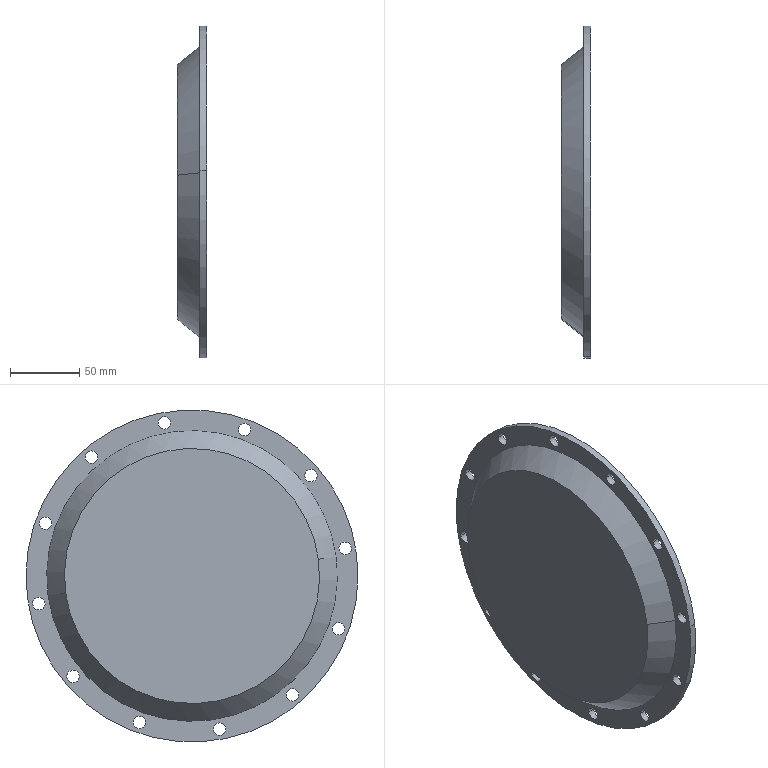Part | NX | features BREP 1 | 1 solid | 34 faces | box 21.199 x 240 x 240 mm | volume 246354 mm3 | cylinder 26 | cone 4 | plane 4 | commonest cylinder face diameters 9 x24 240 x2
STEP:
#1=CARTESIAN_POINT('',(-650.355,90.374,-73.224));
#2=VERTEX_POINT('',#1);
#3=CARTESIAN_POINT('',(-650.355,81.453,-72.035));
#4=VERTEX_POINT('',#3);
#5=CARTESIAN_POINT('',(-650.355,85.914,-72.63));
#6=DIRECTION('',(-1.,0.,0.));
#7=DIRECTION('',(0.,-0.9912,0.1321));
#8=AXIS2_PLACEMENT_3D('',#5,#6,#7);
#9=CIRCLE('',#8,4.5);
#10=EDGE_CURVE('',#2,#4,#9,.T.);
#11=ORIENTED_EDGE('',*,*,#10,.F.);
#12=CARTESIAN_POINT('',(-655.355,90.374,-73.224));
#13=VERTEX_POINT('',#12);
#14=CARTESIAN_POINT('',(-645.355,90.374,-73.224));
#15=DIRECTION('',(1.,0.,0.));
#16=VECTOR('',#15,1000.);
#17=LINE('',#14,#16);
#18=EDGE_CURVE('',#13,#2,#17,.T.);
#19=ORIENTED_EDGE('',*,*,#18,.F.);
#20=CARTESIAN_POINT('',(-655.355,81.453,-72.035));
#21=VERTEX_POINT('',#20);
#22=CARTESIAN_POINT('',(-655.355,85.914,-72.63));
#23=DIRECTION('',(-1.,0.,0.));
#24=DIRECTION('',(0.,-0.9912,0.1321));
#25=AXIS2_PLACEMENT_3D('',#22,#23,#24);
#26=CIRCLE('',#25,4.5);
#27=EDGE_CURVE('',#13,#21,#26,.T.);
#28=ORIENTED_EDGE('',*,*,#27,.T.);
#29=CARTESIAN_POINT('',(-645.355,81.453,-72.035));
#30=DIRECTION('',(1.,0.,0.));
#31=VECTOR('',#30,1000.);
#32=LINE('',#29,#31);
#33=EDGE_CURVE('',#21,#4,#32,.T.);
#34=ORIENTED_EDGE('',*,*,#33,.T.);
#35=EDGE_LOOP('',(#11,#19,#28,#34));
#36=FACE_BOUND('',#35,.T.);
#37=CARTESIAN_POINT('',(-645.355,85.914,-72.63));
#38=DIRECTION('',(-1.,0.,0.));
#39=DIRECTION('',(0.,-0.9912,0.1321));
#40=AXIS2_PLACEMENT_3D('',#37,#38,#39);
#41=CYLINDRICAL_SURFACE('',#40,4.5);
#42=ADVANCED_FACE('',(#36),#41,.F.);
#43=CARTESIAN_POINT('',(-650.355,115.179,-20.537));
#44=VERTEX_POINT('',#43);
#45=CARTESIAN_POINT('',(-650.355,106.258,-19.348));
#46=VERTEX_POINT('',#45);
#47=CARTESIAN_POINT('',(-650.355,110.718,-19.942));
#48=DIRECTION('',(-1.,0.,0.));
#49=DIRECTION('',(0.,-0.9912,0.1321));
#50=AXIS2_PLACEMENT_3D('',#47,#48,#49);
#51=CIRCLE('',#50,4.5);
#52=EDGE_CURVE('',#44,#46,#51,.T.);
#53=ORIENTED_EDGE('',*,*,#52,.F.);
#54=CARTESIAN_POINT('',(-655.355,115.179,-20.537));
#55=VERTEX_POINT('',#54);
#56=CARTESIAN_POINT('',(-645.355,115.179,-20.537));
#57=DIRECTION('',(1.,0.,0.));
#58=VECTOR('',#57,1000.);
#59=LINE('',#56,#58);
#60=EDGE_CURVE('',#55,#44,#59,.T.);
#61=ORIENTED_EDGE('',*,*,#60,.F.);
#62=CARTESIAN_POINT('',(-655.355,106.258,-19.348));
#63=VERTEX_POINT('',#62);
#64=CARTESIAN_POINT('',(-655.355,110.718,-19.942));
#65=DIRECTION('',(-1.,0.,0.));
#66=DIRECTION('',(0.,-0.9912,0.1321));
#67=AXIS2_PLACEMENT_3D('',#64,#65,#66);
#68=CIRCLE('',#67,4.5);
#69=EDGE_CURVE('',#55,#63,#68,.T.);
#70=ORIENTED_EDGE('',*,*,#69,.T.);
#71=CARTESIAN_POINT('',(-645.355,106.258,-19.348));
#72=DIRECTION('',(1.,0.,0.));
#73=VECTOR('',#72,1000.);
#74=LINE('',#71,#73);
#75=EDGE_CURVE('',#63,#46,#74,.T.);
#76=ORIENTED_EDGE('',*,*,#75,.T.);
#77=EDGE_LOOP('',(#53,#61,#70,#76));
#78=FACE_BOUND('',#77,.T.);
#79=CARTESIAN_POINT('',(-645.355,110.718,-19.942));
#80=DIRECTION('',(-1.,0.,0.));
#81=DIRECTION('',(0.,-0.9912,0.1321));
#82=AXIS2_PLACEMENT_3D('',#79,#80,#81);
#83=CYLINDRICAL_SURFACE('',#82,4.5);
#84=ADVANCED_FACE('',(#78),#83,.F.);
#85=CARTESIAN_POINT('',(-650.355,110.317,37.494));
#86=VERTEX_POINT('',#85);
#87=CARTESIAN_POINT('',(-650.355,101.396,38.683));
#88=VERTEX_POINT('',#87);
#89=CARTESIAN_POINT('',(-650.355,105.856,38.088));
#90=DIRECTION('',(-1.,0.,0.));
#91=DIRECTION('',(0.,-0.9912,0.1321));
#92=AXIS2_PLACEMENT_3D('',#89,#90,#91);
#93=CIRCLE('',#92,4.5);
#94=EDGE_CURVE('',#86,#88,#93,.T.);
#95=ORIENTED_EDGE('',*,*,#94,.F.);
#96=CARTESIAN_POINT('',(-655.355,110.317,37.494));
#97=VERTEX_POINT('',#96);
#98=CARTESIAN_POINT('',(-645.355,110.317,37.494));
#99=DIRECTION('',(1.,0.,0.));
#100=VECTOR('',#99,1000.);
#101=LINE('',#98,#100);
#102=EDGE_CURVE('',#97,#86,#101,.T.);
#103=ORIENTED_EDGE('',*,*,#102,.F.);
#104=CARTESIAN_POINT('',(-655.355,101.396,38.683));
#105=VERTEX_POINT('',#104);
#106=CARTESIAN_POINT('',(-655.355,105.856,38.088));
#107=DIRECTION('',(-1.,0.,0.));
#108=DIRECTION('',(0.,-0.9912,0.1321));
#109=AXIS2_PLACEMENT_3D('',#106,#107,#108);
#110=CIRCLE('',#109,4.5);
#111=EDGE_CURVE('',#97,#105,#110,.T.);
#112=ORIENTED_EDGE('',*,*,#111,.T.);
#113=CARTESIAN_POINT('',(-645.355,101.396,38.683));
#114=DIRECTION('',(1.,0.,0.));
#115=VECTOR('',#114,1000.);
#116=LINE('',#113,#115);
#117=EDGE_CURVE('',#105,#88,#116,.T.);
#118=ORIENTED_EDGE('',*,*,#117,.T.);
#119=EDGE_LOOP('',(#95,#103,#112,#118));
#120=FACE_BOUND('',#119,.T.);
#121=CARTESIAN_POINT('',(-645.355,105.856,38.088));
#122=DIRECTION('',(-1.,0.,0.));
#123=DIRECTION('',(0.,-0.9912,0.1321));
#124=AXIS2_PLACEMENT_3D('',#121,#122,#123);
#125=CYLINDRICAL_SURFACE('',#124,4.5);
#126=ADVANCED_FACE('',(#120),#125,.F.);
#127=CARTESIAN_POINT('',(-650.355,77.09,85.319));
#128=VERTEX_POINT('',#127);
#129=CARTESIAN_POINT('',(-650.355,68.169,86.508));
#130=VERTEX_POINT('',#129);
#131=CARTESIAN_POINT('',(-650.355,72.63,85.914));
#132=DIRECTION('',(-1.,0.,0.));
#133=DIRECTION('',(0.,-0.9912,0.1321));
#134=AXIS2_PLACEMENT_3D('',#131,#132,#133);
#135=CIRCLE('',#134,4.5);
#136=EDGE_CURVE('',#128,#130,#135,.T.);
#137=ORIENTED_EDGE('',*,*,#136,.F.);
#138=CARTESIAN_POINT('',(-655.355,77.09,85.319));
#139=VERTEX_POINT('',#138);
#140=CARTESIAN_POINT('',(-645.355,77.09,85.319));
#141=DIRECTION('',(1.,0.,0.));
#142=VECTOR('',#141,1000.);
#143=LINE('',#140,#142);
#144=EDGE_CURVE('',#139,#128,#143,.T.);
#145=ORIENTED_EDGE('',*,*,#144,.F.);
#146=CARTESIAN_POINT('',(-655.355,68.169,86.508));
#147=VERTEX_POINT('',#146);
#148=CARTESIAN_POINT('',(-655.355,72.63,85.914));
#149=DIRECTION('',(-1.,0.,0.));
#150=DIRECTION('',(0.,-0.9912,0.1321));
#151=AXIS2_PLACEMENT_3D('',#148,#149,#150);
#152=CIRCLE('',#151,4.5);
#153=EDGE_CURVE('',#139,#147,#152,.T.);
#154=ORIENTED_EDGE('',*,*,#153,.T.);
#155=CARTESIAN_POINT('',(-645.355,68.169,86.508));
#156=DIRECTION('',(1.,0.,0.));
#157=VECTOR('',#156,1000.);
#158=LINE('',#155,#157);
#159=EDGE_CURVE('',#147,#130,#158,.T.);
#160=ORIENTED_EDGE('',*,*,#159,.T.);
#161=EDGE_LOOP('',(#137,#145,#154,#160));
#162=FACE_BOUND('',#161,.T.);
#163=CARTESIAN_POINT('',(-645.355,72.63,85.914));
#164=DIRECTION('',(-1.,0.,0.));
#165=DIRECTION('',(0.,-0.9912,0.1321));
#166=AXIS2_PLACEMENT_3D('',#163,#164,#165);
#167=CYLINDRICAL_SURFACE('',#166,4.5);
#168=ADVANCED_FACE('',(#162),#167,.F.);
#169=CARTESIAN_POINT('',(-650.355,24.403,110.124));
#170=VERTEX_POINT('',#169);
#171=CARTESIAN_POINT('',(-650.355,15.482,111.313));
#172=VERTEX_POINT('',#171);
#173=CARTESIAN_POINT('',(-650.355,19.942,110.718));
#174=DIRECTION('',(-1.,0.,0.));
#175=DIRECTION('',(0.,-0.9912,0.1321));
#176=AXIS2_PLACEMENT_3D('',#173,#174,#175);
#177=CIRCLE('',#176,4.5);
#178=EDGE_CURVE('',#170,#172,#177,.T.);
#179=ORIENTED_EDGE('',*,*,#178,.F.);
#180=CARTESIAN_POINT('',(-655.355,24.403,110.124));
#181=VERTEX_POINT('',#180);
#182=CARTESIAN_POINT('',(-645.355,24.403,110.124));
#183=DIRECTION('',(1.,0.,0.));
#184=VECTOR('',#183,1000.);
#185=LINE('',#182,#184);
#186=EDGE_CURVE('',#181,#170,#185,.T.);
#187=ORIENTED_EDGE('',*,*,#186,.F.);
#188=CARTESIAN_POINT('',(-655.355,15.482,111.313));
#189=VERTEX_POINT('',#188);
#190=CARTESIAN_POINT('',(-655.355,19.942,110.718));
#191=DIRECTION('',(-1.,0.,0.));
#192=DIRECTION('',(0.,-0.9912,0.1321));
#193=AXIS2_PLACEMENT_3D('',#190,#191,#192);
#194=CIRCLE('',#193,4.5);
#195=EDGE_CURVE('',#181,#189,#194,.T.);
#196=ORIENTED_EDGE('',*,*,#195,.T.);
#197=CARTESIAN_POINT('',(-645.355,15.482,111.313));
#198=DIRECTION('',(1.,0.,0.));
#199=VECTOR('',#198,1000.);
#200=LINE('',#197,#199);
#201=EDGE_CURVE('',#189,#172,#200,.T.);
#202=ORIENTED_EDGE('',*,*,#201,.T.);
#203=EDGE_LOOP('',(#179,#187,#196,#202));
#204=FACE_BOUND('',#203,.T.);
#205=CARTESIAN_POINT('',(-645.355,19.942,110.718));
#206=DIRECTION('',(-1.,0.,0.));
#207=DIRECTION('',(0.,-0.9912,0.1321));
#208=AXIS2_PLACEMENT_3D('',#205,#206,#207);
#209=CYLINDRICAL_SURFACE('',#208,4.5);
#210=ADVANCED_FACE('',(#204),#209,.F.);
#211=CARTESIAN_POINT('',(-650.355,-33.628,105.262));
#212=VERTEX_POINT('',#211);
#213=CARTESIAN_POINT('',(-650.355,-42.549,106.451));
#214=VERTEX_POINT('',#213);
#215=CARTESIAN_POINT('',(-650.355,-38.088,105.856));
#216=DIRECTION('',(-1.,0.,0.));
#217=DIRECTION('',(0.,-0.9912,0.1321));
#218=AXIS2_PLACEMENT_3D('',#215,#216,#217);
#219=CIRCLE('',#218,4.5);
#220=EDGE_CURVE('',#212,#214,#219,.T.);
#221=ORIENTED_EDGE('',*,*,#220,.F.);
#222=CARTESIAN_POINT('',(-655.355,-33.628,105.262));
#223=VERTEX_POINT('',#222);
#224=CARTESIAN_POINT('',(-645.355,-33.628,105.262));
#225=DIRECTION('',(1.,0.,0.));
#226=VECTOR('',#225,1000.);
#227=LINE('',#224,#226);
#228=EDGE_CURVE('',#223,#212,#227,.T.);
#229=ORIENTED_EDGE('',*,*,#228,.F.);
#230=CARTESIAN_POINT('',(-655.355,-42.549,106.451));
#231=VERTEX_POINT('',#230);
#232=CARTESIAN_POINT('',(-655.355,-38.088,105.856));
#233=DIRECTION('',(-1.,0.,0.));
#234=DIRECTION('',(0.,-0.9912,0.1321));
#235=AXIS2_PLACEMENT_3D('',#232,#233,#234);
#236=CIRCLE('',#235,4.5);
#237=EDGE_CURVE('',#223,#231,#236,.T.);
#238=ORIENTED_EDGE('',*,*,#237,.T.);
#239=CARTESIAN_POINT('',(-645.355,-42.549,106.451));
#240=DIRECTION('',(1.,0.,0.));
#241=VECTOR('',#240,1000.);
#242=LINE('',#239,#241);
#243=EDGE_CURVE('',#231,#214,#242,.T.);
#244=ORIENTED_EDGE('',*,*,#243,.T.);
#245=EDGE_LOOP('',(#221,#229,#238,#244));
#246=FACE_BOUND('',#245,.T.);
#247=CARTESIAN_POINT('',(-645.355,-38.088,105.856));
#248=DIRECTION('',(-1.,0.,0.));
#249=DIRECTION('',(0.,-0.9912,0.1321));
#250=AXIS2_PLACEMENT_3D('',#247,#248,#249);
#251=CYLINDRICAL_SURFACE('',#250,4.5);
#252=ADVANCED_FACE('',(#246),#251,.F.);
#253=CARTESIAN_POINT('',(-650.355,-81.453,72.035));
#254=VERTEX_POINT('',#253);
#255=CARTESIAN_POINT('',(-650.355,-90.374,73.224));
#256=VERTEX_POINT('',#255);
#257=CARTESIAN_POINT('',(-650.355,-85.914,72.63));
#258=DIRECTION('',(-1.,0.,0.));
#259=DIRECTION('',(0.,-0.9912,0.1321));
#260=AXIS2_PLACEMENT_3D('',#257,#258,#259);
#261=CIRCLE('',#260,4.5);
#262=EDGE_CURVE('',#254,#256,#261,.T.);
#263=ORIENTED_EDGE('',*,*,#262,.F.);
#264=CARTESIAN_POINT('',(-655.355,-81.453,72.035));
#265=VERTEX_POINT('',#264);
#266=CARTESIAN_POINT('',(-645.355,-81.453,72.035));
#267=DIRECTION('',(1.,0.,0.));
#268=VECTOR('',#267,1000.);
#269=LINE('',#266,#268);
#270=EDGE_CURVE('',#265,#254,#269,.T.);
#271=ORIENTED_EDGE('',*,*,#270,.F.);
#272=CARTESIAN_POINT('',(-655.355,-90.374,73.224));
#273=VERTEX_POINT('',#272);
#274=CARTESIAN_POINT('',(-655.355,-85.914,72.63));
#275=DIRECTION('',(-1.,0.,0.));
#276=DIRECTION('',(0.,-0.9912,0.1321));
#277=AXIS2_PLACEMENT_3D('',#274,#275,#276);
#278=CIRCLE('',#277,4.5);
#279=EDGE_CURVE('',#265,#273,#278,.T.);
#280=ORIENTED_EDGE('',*,*,#279,.T.);
#281=CARTESIAN_POINT('',(-645.355,-90.374,73.224));
#282=DIRECTION('',(1.,0.,0.));
#283=VECTOR('',#282,1000.);
#284=LINE('',#281,#283);
#285=EDGE_CURVE('',#273,#256,#284,.T.);
#286=ORIENTED_EDGE('',*,*,#285,.T.);
#287=EDGE_LOOP('',(#263,#271,#280,#286));
#288=FACE_BOUND('',#287,.T.);
#289=CARTESIAN_POINT('',(-645.355,-85.914,72.63));
#290=DIRECTION('',(-1.,0.,0.));
#291=DIRECTION('',(0.,-0.9912,0.1321));
#292=AXIS2_PLACEMENT_3D('',#289,#290,#291);
#293=CYLINDRICAL_SURFACE('',#292,4.5);
#294=ADVANCED_FACE('',(#288),#293,.F.);
#295=CARTESIAN_POINT('',(-650.355,-106.258,19.348));
#296=VERTEX_POINT('',#295);
#297=CARTESIAN_POINT('',(-650.355,-115.179,20.537));
#298=VERTEX_POINT('',#297);
#299=CARTESIAN_POINT('',(-650.355,-110.718,19.942));
#300=DIRECTION('',(-1.,0.,0.));
#301=DIRECTION('',(0.,-0.9912,0.1321));
#302=AXIS2_PLACEMENT_3D('',#299,#300,#301);
#303=CIRCLE('',#302,4.5);
#304=EDGE_CURVE('',#296,#298,#303,.T.);
#305=ORIENTED_EDGE('',*,*,#304,.F.);
#306=CARTESIAN_POINT('',(-655.355,-106.258,19.348));
#307=VERTEX_POINT('',#306);
#308=CARTESIAN_POINT('',(-645.355,-106.258,19.348));
#309=DIRECTION('',(1.,0.,0.));
#310=VECTOR('',#309,1000.);
#311=LINE('',#308,#310);
#312=EDGE_CURVE('',#307,#296,#311,.T.);
#313=ORIENTED_EDGE('',*,*,#312,.F.);
#314=CARTESIAN_POINT('',(-655.355,-115.179,20.537));
#315=VERTEX_POINT('',#314);
#316=CARTESIAN_POINT('',(-655.355,-110.718,19.942));
#317=DIRECTION('',(-1.,0.,0.));
#318=DIRECTION('',(0.,-0.9912,0.1321));
#319=AXIS2_PLACEMENT_3D('',#316,#317,#318);
#320=CIRCLE('',#319,4.5);
#321=EDGE_CURVE('',#307,#315,#320,.T.);
#322=ORIENTED_EDGE('',*,*,#321,.T.);
#323=CARTESIAN_POINT('',(-645.355,-115.179,20.537));
#324=DIRECTION('',(1.,0.,0.));
#325=VECTOR('',#324,1000.);
#326=LINE('',#323,#325);
#327=EDGE_CURVE('',#315,#298,#326,.T.);
#328=ORIENTED_EDGE('',*,*,#327,.T.);
#329=EDGE_LOOP('',(#305,#313,#322,#328));
#330=FACE_BOUND('',#329,.T.);
#331=CARTESIAN_POINT('',(-645.355,-110.718,19.942));
#332=DIRECTION('',(-1.,0.,0.));
#333=DIRECTION('',(0.,-0.9912,0.1321));
#334=AXIS2_PLACEMENT_3D('',#331,#332,#333);
#335=CYLINDRICAL_SURFACE('',#334,4.5);
#336=ADVANCED_FACE('',(#330),#335,.F.);
#337=CARTESIAN_POINT('',(-650.355,-101.396,-38.683));
#338=VERTEX_POINT('',#337);
#339=CARTESIAN_POINT('',(-650.355,-110.317,-37.494));
#340=VERTEX_POINT('',#339);
#341=CARTESIAN_POINT('',(-650.355,-105.856,-38.088));
#342=DIRECTION('',(-1.,0.,0.));
#343=DIRECTION('',(0.,-0.9912,0.1321));
#344=AXIS2_PLACEMENT_3D('',#341,#342,#343);
#345=CIRCLE('',#344,4.5);
#346=EDGE_CURVE('',#338,#340,#345,.T.);
#347=ORIENTED_EDGE('',*,*,#346,.F.);
#348=CARTESIAN_POINT('',(-655.355,-101.396,-38.683));
#349=VERTEX_POINT('',#348);
#350=CARTESIAN_POINT('',(-645.355,-101.396,-38.683));
#351=DIRECTION('',(1.,0.,0.));
#352=VECTOR('',#351,1000.);
#353=LINE('',#350,#352);
#354=EDGE_CURVE('',#349,#338,#353,.T.);
#355=ORIENTED_EDGE('',*,*,#354,.F.);
#356=CARTESIAN_POINT('',(-655.355,-110.317,-37.494));
#357=VERTEX_POINT('',#356);
#358=CARTESIAN_POINT('',(-655.355,-105.856,-38.088));
#359=DIRECTION('',(-1.,0.,0.));
#360=DIRECTION('',(0.,-0.9912,0.1321));
#361=AXIS2_PLACEMENT_3D('',#358,#359,#360);
#362=CIRCLE('',#361,4.5);
#363=EDGE_CURVE('',#349,#357,#362,.T.);
#364=ORIENTED_EDGE('',*,*,#363,.T.);
#365=CARTESIAN_POINT('',(-645.355,-110.317,-37.494));
#366=DIRECTION('',(1.,0.,0.));
#367=VECTOR('',#366,1000.);
#368=LINE('',#365,#367);
#369=EDGE_CURVE('',#357,#340,#368,.T.);
#370=ORIENTED_EDGE('',*,*,#369,.T.);
#371=EDGE_LOOP('',(#347,#355,#364,#370));
#372=FACE_BOUND('',#371,.T.);
#373=CARTESIAN_POINT('',(-645.355,-105.856,-38.088));
#374=DIRECTION('',(-1.,0.,0.));
#375=DIRECTION('',(0.,-0.9912,0.1321));
#376=AXIS2_PLACEMENT_3D('',#373,#374,#375);
#377=CYLINDRICAL_SURFACE('',#376,4.5);
#378=ADVANCED_FACE('',(#372),#377,.F.);
#379=CARTESIAN_POINT('',(-650.355,-68.169,-86.508));
#380=VERTEX_POINT('',#379);
#381=CARTESIAN_POINT('',(-650.355,-77.09,-85.319));
#382=VERTEX_POINT('',#381);
#383=CARTESIAN_POINT('',(-650.355,-72.63,-85.914));
#384=DIRECTION('',(-1.,0.,0.));
#385=DIRECTION('',(0.,-0.9912,0.1321));
#386=AXIS2_PLACEMENT_3D('',#383,#384,#385);
#387=CIRCLE('',#386,4.5);
#388=EDGE_CURVE('',#380,#382,#387,.T.);
#389=ORIENTED_EDGE('',*,*,#388,.F.);
#390=CARTESIAN_POINT('',(-655.355,-68.169,-86.508));
#391=VERTEX_POINT('',#390);
#392=CARTESIAN_POINT('',(-645.355,-68.169,-86.508));
#393=DIRECTION('',(1.,0.,0.));
#394=VECTOR('',#393,1000.);
#395=LINE('',#392,#394);
#396=EDGE_CURVE('',#391,#380,#395,.T.);
#397=ORIENTED_EDGE('',*,*,#396,.F.);
#398=CARTESIAN_POINT('',(-655.355,-77.09,-85.319));
#399=VERTEX_POINT('',#398);
#400=CARTESIAN_POINT('',(-655.355,-72.63,-85.914));
#401=DIRECTION('',(-1.,0.,0.));
#402=DIRECTION('',(0.,-0.9912,0.1321));
#403=AXIS2_PLACEMENT_3D('',#400,#401,#402);
#404=CIRCLE('',#403,4.5);
#405=EDGE_CURVE('',#391,#399,#404,.T.);
#406=ORIENTED_EDGE('',*,*,#405,.T.);
#407=CARTESIAN_POINT('',(-645.355,-77.09,-85.319));
#408=DIRECTION('',(1.,0.,0.));
#409=VECTOR('',#408,1000.);
#410=LINE('',#407,#409);
#411=EDGE_CURVE('',#399,#382,#410,.T.);
#412=ORIENTED_EDGE('',*,*,#411,.T.);
#413=EDGE_LOOP('',(#389,#397,#406,#412));
#414=FACE_BOUND('',#413,.T.);
#415=CARTESIAN_POINT('',(-645.355,-72.63,-85.914));
#416=DIRECTION('',(-1.,0.,0.));
#417=DIRECTION('',(0.,-0.9912,0.1321));
#418=AXIS2_PLACEMENT_3D('',#415,#416,#417);
#419=CYLINDRICAL_SURFACE('',#418,4.5);
#420=ADVANCED_FACE('',(#414),#419,.F.);
#421=CARTESIAN_POINT('',(-650.355,-15.482,-111.313));
#422=VERTEX_POINT('',#421);
#423=CARTESIAN_POINT('',(-650.355,-24.403,-110.124));
#424=VERTEX_POINT('',#423);
#425=CARTESIAN_POINT('',(-650.355,-19.942,-110.718));
#426=DIRECTION('',(-1.,0.,0.));
#427=DIRECTION('',(0.,-0.9912,0.1321));
#428=AXIS2_PLACEMENT_3D('',#425,#426,#427);
#429=CIRCLE('',#428,4.5);
#430=EDGE_CURVE('',#422,#424,#429,.T.);
#431=ORIENTED_EDGE('',*,*,#430,.F.);
#432=CARTESIAN_POINT('',(-655.355,-15.482,-111.313));
#433=VERTEX_POINT('',#432);
#434=CARTESIAN_POINT('',(-645.355,-15.482,-111.313));
#435=DIRECTION('',(1.,0.,0.));
#436=VECTOR('',#435,1000.);
#437=LINE('',#434,#436);
#438=EDGE_CURVE('',#433,#422,#437,.T.);
#439=ORIENTED_EDGE('',*,*,#438,.F.);
#440=CARTESIAN_POINT('',(-655.355,-24.403,-110.124));
#441=VERTEX_POINT('',#440);
#442=CARTESIAN_POINT('',(-655.355,-19.942,-110.718));
#443=DIRECTION('',(-1.,0.,0.));
#444=DIRECTION('',(0.,-0.9912,0.1321));
#445=AXIS2_PLACEMENT_3D('',#442,#443,#444);
#446=CIRCLE('',#445,4.5);
#447=EDGE_CURVE('',#433,#441,#446,.T.);
#448=ORIENTED_EDGE('',*,*,#447,.T.);
#449=CARTESIAN_POINT('',(-645.355,-24.403,-110.124));
#450=DIRECTION('',(1.,0.,0.));
#451=VECTOR('',#450,1000.);
#452=LINE('',#449,#451);
#453=EDGE_CURVE('',#441,#424,#452,.T.);
#454=ORIENTED_EDGE('',*,*,#453,.T.);
#455=EDGE_LOOP('',(#431,#439,#448,#454));
#456=FACE_BOUND('',#455,.T.);
#457=CARTESIAN_POINT('',(-645.355,-19.942,-110.718));
#458=DIRECTION('',(-1.,0.,0.));
#459=DIRECTION('',(0.,-0.9912,0.1321));
#460=AXIS2_PLACEMENT_3D('',#457,#458,#459);
#461=CYLINDRICAL_SURFACE('',#460,4.5);
#462=ADVANCED_FACE('',(#456),#461,.F.);
#463=CARTESIAN_POINT('',(-650.355,42.549,-106.451));
#464=VERTEX_POINT('',#463);
#465=CARTESIAN_POINT('',(-650.355,33.628,-105.262));
#466=VERTEX_POINT('',#465);
#467=CARTESIAN_POINT('',(-650.355,38.088,-105.856));
#468=DIRECTION('',(-1.,0.,0.));
#469=DIRECTION('',(0.,-0.9912,0.1321));
#470=AXIS2_PLACEMENT_3D('',#467,#468,#469);
#471=CIRCLE('',#470,4.5);
#472=EDGE_CURVE('',#464,#466,#471,.T.);
#473=ORIENTED_EDGE('',*,*,#472,.F.);
#474=CARTESIAN_POINT('',(-655.355,42.549,-106.451));
#475=VERTEX_POINT('',#474);
#476=CARTESIAN_POINT('',(-645.355,42.549,-106.451));
#477=DIRECTION('',(1.,0.,0.));
#478=VECTOR('',#477,1000.);
#479=LINE('',#476,#478);
#480=EDGE_CURVE('',#475,#464,#479,.T.);
#481=ORIENTED_EDGE('',*,*,#480,.F.);
#482=CARTESIAN_POINT('',(-655.355,33.628,-105.262));
#483=VERTEX_POINT('',#482);
#484=CARTESIAN_POINT('',(-655.355,38.088,-105.856));
#485=DIRECTION('',(-1.,0.,0.));
#486=DIRECTION('',(0.,-0.9912,0.1321));
#487=AXIS2_PLACEMENT_3D('',#484,#485,#486);
#488=CIRCLE('',#487,4.5);
#489=EDGE_CURVE('',#475,#483,#488,.T.);
#490=ORIENTED_EDGE('',*,*,#489,.T.);
#491=CARTESIAN_POINT('',(-645.355,33.628,-105.262));
#492=DIRECTION('',(1.,0.,0.));
#493=VECTOR('',#492,1000.);
#494=LINE('',#491,#493);
#495=EDGE_CURVE('',#483,#466,#494,.T.);
#496=ORIENTED_EDGE('',*,*,#495,.T.);
#497=EDGE_LOOP('',(#473,#481,#490,#496));
#498=FACE_BOUND('',#497,.T.);
#499=CARTESIAN_POINT('',(-645.355,38.088,-105.856));
#500=DIRECTION('',(-1.,0.,0.));
#501=DIRECTION('',(0.,-0.9912,0.1321));
#502=AXIS2_PLACEMENT_3D('',#499,#500,#501);
#503=CYLINDRICAL_SURFACE('',#502,4.5);
#504=ADVANCED_FACE('',(#498),#503,.F.);
#505=CARTESIAN_POINT('',(-671.554,-91.37,12.178));
#506=VERTEX_POINT('',#505);
#507=CARTESIAN_POINT('',(-671.554,91.37,-12.178));
#508=VERTEX_POINT('',#507);
#509=CARTESIAN_POINT('',(-671.554,0.,0.));
#510=DIRECTION('',(-1.,0.,0.));
#511=DIRECTION('',(0.,-0.9912,0.1321));
#512=AXIS2_PLACEMENT_3D('',#509,#510,#511);
#513=CIRCLE('',#512,92.178);
#514=EDGE_CURVE('',#506,#508,#513,.T.);
#515=ORIENTED_EDGE('',*,*,#514,.F.);
#516=CARTESIAN_POINT('',(-655.355,-104.08,13.872));
#517=VERTEX_POINT('',#516);
#518=CARTESIAN_POINT('',(-655.355,-104.08,13.872));
#519=DIRECTION('',(-0.7841,0.6152,-0.082));
#520=VECTOR('',#519,1000.);
#521=LINE('',#518,#520);
#522=EDGE_CURVE('',#506,#517,#521,.F.);
#523=ORIENTED_EDGE('',*,*,#522,.T.);
#524=CARTESIAN_POINT('',(-655.355,104.08,-13.872));
#525=VERTEX_POINT('',#524);
#526=CARTESIAN_POINT('',(-655.355,0.,0.));
#527=DIRECTION('',(-1.,0.,0.));
#528=DIRECTION('',(0.,-0.9912,0.1321));
#529=AXIS2_PLACEMENT_3D('',#526,#527,#528);
#530=CIRCLE('',#529,105.);
#531=EDGE_CURVE('',#517,#525,#530,.T.);
#532=ORIENTED_EDGE('',*,*,#531,.T.);
#533=CARTESIAN_POINT('',(-655.355,104.08,-13.872));
#534=DIRECTION('',(-0.7841,-0.6152,0.082));
#535=VECTOR('',#534,1000.);
#536=LINE('',#533,#535);
#537=EDGE_CURVE('',#508,#525,#536,.F.);
#538=ORIENTED_EDGE('',*,*,#537,.F.);
#539=EDGE_LOOP('',(#515,#523,#532,#538));
#540=FACE_BOUND('',#539,.T.);
#541=CARTESIAN_POINT('',(-655.355,0.,0.));
#542=DIRECTION('',(1.,0.,0.));
#543=DIRECTION('',(0.,0.9912,-0.1321));
#544=AXIS2_PLACEMENT_3D('',#541,#542,#543);
#545=CONICAL_SURFACE('',#544,105.,0.6696);
#546=ADVANCED_FACE('',(#540),#545,.T.);
#547=CARTESIAN_POINT('',(-650.355,-118.948,15.854));
#548=VERTEX_POINT('',#547);
#549=CARTESIAN_POINT('',(-650.355,118.948,-15.854));
#550=VERTEX_POINT('',#549);
#551=CARTESIAN_POINT('',(-650.355,0.,0.));
#552=DIRECTION('',(-1.,0.,0.));
#553=DIRECTION('',(0.,-0.9912,0.1321));
#554=AXIS2_PLACEMENT_3D('',#551,#552,#553);
#555=CIRCLE('',#554,120.);
#556=EDGE_CURVE('',#548,#550,#555,.T.);
#557=ORIENTED_EDGE('',*,*,#556,.T.);
#558=CARTESIAN_POINT('',(-655.355,118.948,-15.854));
#559=VERTEX_POINT('',#558);
#560=CARTESIAN_POINT('',(-671.554,118.948,-15.854));
#561=DIRECTION('',(1.,0.,0.));
#562=VECTOR('',#561,1000.);
#563=LINE('',#560,#562);
#564=EDGE_CURVE('',#559,#550,#563,.T.);
#565=ORIENTED_EDGE('',*,*,#564,.F.);
#566=CARTESIAN_POINT('',(-655.355,-118.948,15.854));
#567=VERTEX_POINT('',#566);
#568=CARTESIAN_POINT('',(-655.355,0.,0.));
#569=DIRECTION('',(-1.,0.,0.));
#570=DIRECTION('',(0.,-0.9912,0.1321));
#571=AXIS2_PLACEMENT_3D('',#568,#569,#570);
#572=CIRCLE('',#571,120.);
#573=EDGE_CURVE('',#567,#559,#572,.T.);
#574=ORIENTED_EDGE('',*,*,#573,.F.);
#575=CARTESIAN_POINT('',(-671.554,-118.948,15.854));
#576=DIRECTION('',(1.,0.,0.));
#577=VECTOR('',#576,1000.);
#578=LINE('',#575,#577);
#579=EDGE_CURVE('',#567,#548,#578,.T.);
#580=ORIENTED_EDGE('',*,*,#579,.T.);
#581=EDGE_LOOP('',(#557,#565,#574,#580));
#582=FACE_BOUND('',#581,.T.);
#583=CARTESIAN_POINT('',(-671.554,0.,0.));
#584=DIRECTION('',(-1.,0.,0.));
#585=DIRECTION('',(0.,-0.9912,0.1321));
#586=AXIS2_PLACEMENT_3D('',#583,#584,#585);
#587=CYLINDRICAL_SURFACE('',#586,120.);
#588=ADVANCED_FACE('',(#582),#587,.T.);
#589=CARTESIAN_POINT('',(-666.554,88.972,-11.858));
#590=VERTEX_POINT('',#589);
#591=CARTESIAN_POINT('',(-666.554,-88.972,11.858));
#592=VERTEX_POINT('',#591);
#593=CARTESIAN_POINT('',(-666.554,0.,0.));
#594=DIRECTION('',(-1.,0.,0.));
#595=DIRECTION('',(0.,-0.9912,0.1321));
#596=AXIS2_PLACEMENT_3D('',#593,#594,#595);
#597=CIRCLE('',#596,89.759);
#598=EDGE_CURVE('',#590,#592,#597,.T.);
#599=ORIENTED_EDGE('',*,*,#598,.T.);
#600=CARTESIAN_POINT('',(-650.355,-101.682,13.552));
#601=VERTEX_POINT('',#600);
#602=CARTESIAN_POINT('',(-666.554,-88.972,11.858));
#603=DIRECTION('',(-0.7841,0.6152,-0.082));
#604=VECTOR('',#603,1000.);
#605=LINE('',#602,#604);
#606=EDGE_CURVE('',#592,#601,#605,.F.);
#607=ORIENTED_EDGE('',*,*,#606,.T.);
#608=CARTESIAN_POINT('',(-650.355,101.682,-13.552));
#609=VERTEX_POINT('',#608);
#610=CARTESIAN_POINT('',(-650.355,0.,0.));
#611=DIRECTION('',(-1.,0.,0.));
#612=DIRECTION('',(0.,-0.9912,0.1321));
#613=AXIS2_PLACEMENT_3D('',#610,#611,#612);
#614=CIRCLE('',#613,102.581);
#615=EDGE_CURVE('',#609,#601,#614,.T.);
#616=ORIENTED_EDGE('',*,*,#615,.F.);
#617=CARTESIAN_POINT('',(-666.554,88.972,-11.858));
#618=DIRECTION('',(-0.7841,-0.6152,0.082));
#619=VECTOR('',#618,1000.);
#620=LINE('',#617,#619);
#621=EDGE_CURVE('',#590,#609,#620,.F.);
#622=ORIENTED_EDGE('',*,*,#621,.F.);
#623=EDGE_LOOP('',(#599,#607,#616,#622));
#624=FACE_BOUND('',#623,.T.);
#625=CARTESIAN_POINT('',(-666.554,0.,0.));
#626=DIRECTION('',(1.,0.,0.));
#627=DIRECTION('',(0.,0.9912,-0.1321));
#628=AXIS2_PLACEMENT_3D('',#625,#626,#627);
#629=CONICAL_SURFACE('',#628,89.759,0.6696);
#630=ADVANCED_FACE('',(#624),#629,.F.);
#631=CARTESIAN_POINT('',(-671.554,0.,0.));
#632=DIRECTION('',(-1.,0.,0.));
#633=DIRECTION('',(0.,-0.9912,0.1321));
#634=AXIS2_PLACEMENT_3D('',#631,#632,#633);
#635=CIRCLE('',#634,92.178);
#636=EDGE_CURVE('',#508,#506,#635,.T.);
#637=ORIENTED_EDGE('',*,*,#636,.T.);
#638=ORIENTED_EDGE('',*,*,#514,.T.);
#639=EDGE_LOOP('',(#637,#638));
#640=FACE_BOUND('',#639,.T.);
#641=CARTESIAN_POINT('',(-671.554,91.37,-12.178));
#642=DIRECTION('',(1.,0.,0.));
#643=DIRECTION('',(0.,0.9912,-0.1321));
#644=AXIS2_PLACEMENT_3D('',#641,#642,#643);
#645=PLANE('',#644);
#646=ADVANCED_FACE('',(#640),#645,.F.);
#647=ORIENTED_EDGE('',*,*,#598,.F.);
#648=CARTESIAN_POINT('',(-666.554,0.,0.));
#649=DIRECTION('',(-1.,0.,0.));
#650=DIRECTION('',(0.,-0.9912,0.1321));
#651=AXIS2_PLACEMENT_3D('',#648,#649,#650);
#652=CIRCLE('',#651,89.759);
#653=EDGE_CURVE('',#592,#590,#652,.T.);
#654=ORIENTED_EDGE('',*,*,#653,.F.);
#655=EDGE_LOOP('',(#647,#654));
#656=FACE_BOUND('',#655,.T.);
#657=CARTESIAN_POINT('',(-666.554,0.,0.));
#658=DIRECTION('',(-1.,0.,0.));
#659=DIRECTION('',(0.,-0.9912,0.1321));
#660=AXIS2_PLACEMENT_3D('',#657,#658,#659);
#661=PLANE('',#660);
#662=ADVANCED_FACE('',(#656),#661,.F.);
#663=ORIENTED_EDGE('',*,*,#606,.F.);
#664=ORIENTED_EDGE('',*,*,#653,.T.);
#665=ORIENTED_EDGE('',*,*,#621,.T.);
#666=CARTESIAN_POINT('',(-650.355,0.,0.));
#667=DIRECTION('',(-1.,0.,0.));
#668=DIRECTION('',(0.,-0.9912,0.1321));
#669=AXIS2_PLACEMENT_3D('',#666,#667,#668);
#670=CIRCLE('',#669,102.581);
#671=EDGE_CURVE('',#601,#609,#670,.T.);
#672=ORIENTED_EDGE('',*,*,#671,.F.);
#673=EDGE_LOOP('',(#663,#664,#665,#672));
#674=FACE_BOUND('',#673,.T.);
#675=CARTESIAN_POINT('',(-666.554,0.,0.));
#676=DIRECTION('',(1.,0.,0.));
#677=DIRECTION('',(0.,0.9912,-0.1321));
#678=AXIS2_PLACEMENT_3D('',#675,#676,#677);
#679=CONICAL_SURFACE('',#678,89.759,0.6696);
#680=ADVANCED_FACE('',(#674),#679,.F.);
#681=CARTESIAN_POINT('',(-650.355,85.914,-72.63));
#682=DIRECTION('',(-1.,0.,0.));
#683=DIRECTION('',(0.,-0.9912,0.1321));
#684=AXIS2_PLACEMENT_3D('',#681,#682,#683);
#685=CIRCLE('',#684,4.5);
#686=EDGE_CURVE('',#4,#2,#685,.T.);
#687=ORIENTED_EDGE('',*,*,#686,.T.);
#688=ORIENTED_EDGE('',*,*,#10,.T.);
#689=EDGE_LOOP('',(#687,#688));
#690=FACE_BOUND('',#689,.T.);
#691=CARTESIAN_POINT('',(-650.355,110.718,-19.942));
#692=DIRECTION('',(-1.,0.,0.));
#693=DIRECTION('',(0.,-0.9912,0.1321));
#694=AXIS2_PLACEMENT_3D('',#691,#692,#693);
#695=CIRCLE('',#694,4.5);
#696=EDGE_CURVE('',#46,#44,#695,.T.);
#697=ORIENTED_EDGE('',*,*,#696,.T.);
#698=ORIENTED_EDGE('',*,*,#52,.T.);
#699=EDGE_LOOP('',(#697,#698));
#700=FACE_BOUND('',#699,.T.);
#701=CARTESIAN_POINT('',(-650.355,105.856,38.088));
#702=DIRECTION('',(-1.,0.,0.));
#703=DIRECTION('',(0.,-0.9912,0.1321));
#704=AXIS2_PLACEMENT_3D('',#701,#702,#703);
#705=CIRCLE('',#704,4.5);
#706=EDGE_CURVE('',#88,#86,#705,.T.);
#707=ORIENTED_EDGE('',*,*,#706,.T.);
#708=ORIENTED_EDGE('',*,*,#94,.T.);
#709=EDGE_LOOP('',(#707,#708));
#710=FACE_BOUND('',#709,.T.);
#711=CARTESIAN_POINT('',(-650.355,72.63,85.914));
#712=DIRECTION('',(-1.,0.,0.));
#713=DIRECTION('',(0.,-0.9912,0.1321));
#714=AXIS2_PLACEMENT_3D('',#711,#712,#713);
#715=CIRCLE('',#714,4.5);
#716=EDGE_CURVE('',#130,#128,#715,.T.);
#717=ORIENTED_EDGE('',*,*,#716,.T.);
#718=ORIENTED_EDGE('',*,*,#136,.T.);
#719=EDGE_LOOP('',(#717,#718));
#720=FACE_BOUND('',#719,.T.);
#721=CARTESIAN_POINT('',(-650.355,19.942,110.718));
#722=DIRECTION('',(-1.,0.,0.));
#723=DIRECTION('',(0.,-0.9912,0.1321));
#724=AXIS2_PLACEMENT_3D('',#721,#722,#723);
#725=CIRCLE('',#724,4.5);
#726=EDGE_CURVE('',#172,#170,#725,.T.);
#727=ORIENTED_EDGE('',*,*,#726,.T.);
#728=ORIENTED_EDGE('',*,*,#178,.T.);
#729=EDGE_LOOP('',(#727,#728));
#730=FACE_BOUND('',#729,.T.);
#731=CARTESIAN_POINT('',(-650.355,-38.088,105.856));
#732=DIRECTION('',(-1.,0.,0.));
#733=DIRECTION('',(0.,-0.9912,0.1321));
#734=AXIS2_PLACEMENT_3D('',#731,#732,#733);
#735=CIRCLE('',#734,4.5);
#736=EDGE_CURVE('',#214,#212,#735,.T.);
#737=ORIENTED_EDGE('',*,*,#736,.T.);
#738=ORIENTED_EDGE('',*,*,#220,.T.);
#739=EDGE_LOOP('',(#737,#738));
#740=FACE_BOUND('',#739,.T.);
#741=CARTESIAN_POINT('',(-650.355,-85.914,72.63));
#742=DIRECTION('',(-1.,0.,0.));
#743=DIRECTION('',(0.,-0.9912,0.1321));
#744=AXIS2_PLACEMENT_3D('',#741,#742,#743);
#745=CIRCLE('',#744,4.5);
#746=EDGE_CURVE('',#256,#254,#745,.T.);
#747=ORIENTED_EDGE('',*,*,#746,.T.);
#748=ORIENTED_EDGE('',*,*,#262,.T.);
#749=EDGE_LOOP('',(#747,#748));
#750=FACE_BOUND('',#749,.T.);
#751=CARTESIAN_POINT('',(-650.355,-110.718,19.942));
#752=DIRECTION('',(-1.,0.,0.));
#753=DIRECTION('',(0.,-0.9912,0.1321));
#754=AXIS2_PLACEMENT_3D('',#751,#752,#753);
#755=CIRCLE('',#754,4.5);
#756=EDGE_CURVE('',#298,#296,#755,.T.);
#757=ORIENTED_EDGE('',*,*,#756,.T.);
#758=ORIENTED_EDGE('',*,*,#304,.T.);
#759=EDGE_LOOP('',(#757,#758));
#760=FACE_BOUND('',#759,.T.);
#761=CARTESIAN_POINT('',(-650.355,-105.856,-38.088));
#762=DIRECTION('',(-1.,0.,0.));
#763=DIRECTION('',(0.,-0.9912,0.1321));
#764=AXIS2_PLACEMENT_3D('',#761,#762,#763);
#765=CIRCLE('',#764,4.5);
#766=EDGE_CURVE('',#340,#338,#765,.T.);
#767=ORIENTED_EDGE('',*,*,#766,.T.);
#768=ORIENTED_EDGE('',*,*,#346,.T.);
#769=EDGE_LOOP('',(#767,#768));
#770=FACE_BOUND('',#769,.T.);
#771=CARTESIAN_POINT('',(-650.355,-72.63,-85.914));
#772=DIRECTION('',(-1.,0.,0.));
#773=DIRECTION('',(0.,-0.9912,0.1321));
#774=AXIS2_PLACEMENT_3D('',#771,#772,#773);
#775=CIRCLE('',#774,4.5);
#776=EDGE_CURVE('',#382,#380,#775,.T.);
#777=ORIENTED_EDGE('',*,*,#776,.T.);
#778=ORIENTED_EDGE('',*,*,#388,.T.);
#779=EDGE_LOOP('',(#777,#778));
#780=FACE_BOUND('',#779,.T.);
#781=CARTESIAN_POINT('',(-650.355,-19.942,-110.718));
#782=DIRECTION('',(-1.,0.,0.));
#783=DIRECTION('',(0.,-0.9912,0.1321));
#784=AXIS2_PLACEMENT_3D('',#781,#782,#783);
#785=CIRCLE('',#784,4.5);
#786=EDGE_CURVE('',#424,#422,#785,.T.);
#787=ORIENTED_EDGE('',*,*,#786,.T.);
#788=ORIENTED_EDGE('',*,*,#430,.T.);
#789=EDGE_LOOP('',(#787,#788));
#790=FACE_BOUND('',#789,.T.);
#791=CARTESIAN_POINT('',(-650.355,38.088,-105.856));
#792=DIRECTION('',(-1.,0.,0.));
#793=DIRECTION('',(0.,-0.9912,0.1321));
#794=AXIS2_PLACEMENT_3D('',#791,#792,#793);
#795=CIRCLE('',#794,4.5);
#796=EDGE_CURVE('',#466,#464,#795,.T.);
#797=ORIENTED_EDGE('',*,*,#796,.T.);
#798=ORIENTED_EDGE('',*,*,#472,.T.);
#799=EDGE_LOOP('',(#797,#798));
#800=FACE_BOUND('',#799,.T.);
#801=ORIENTED_EDGE('',*,*,#556,.F.);
#802=CARTESIAN_POINT('',(-650.355,0.,0.));
#803=DIRECTION('',(-1.,0.,0.));
#804=DIRECTION('',(0.,-0.9912,0.1321));
#805=AXIS2_PLACEMENT_3D('',#802,#803,#804);
#806=CIRCLE('',#805,120.);
#807=EDGE_CURVE('',#550,#548,#806,.T.);
#808=ORIENTED_EDGE('',*,*,#807,.F.);
#809=EDGE_LOOP('',(#801,#808));
#810=FACE_BOUND('',#809,.T.);
#811=ORIENTED_EDGE('',*,*,#615,.T.);
#812=ORIENTED_EDGE('',*,*,#671,.T.);
#813=EDGE_LOOP('',(#811,#812));
#814=FACE_BOUND('',#813,.T.);
#815=CARTESIAN_POINT('',(-650.355,101.682,-13.552));
#816=DIRECTION('',(-1.,0.,0.));
#817=DIRECTION('',(0.,-0.9912,0.1321));
#818=AXIS2_PLACEMENT_3D('',#815,#816,#817);
#819=PLANE('',#818);
#820=ADVANCED_FACE('',(#690,#700,#710,#720,#730,#740,#750,#760,#770,#780,#790,#800,#810,#814),#819,.F.);
#821=ORIENTED_EDGE('',*,*,#564,.T.);
#822=ORIENTED_EDGE('',*,*,#807,.T.);
#823=ORIENTED_EDGE('',*,*,#579,.F.);
#824=CARTESIAN_POINT('',(-655.355,0.,0.));
#825=DIRECTION('',(-1.,0.,0.));
#826=DIRECTION('',(0.,-0.9912,0.1321));
#827=AXIS2_PLACEMENT_3D('',#824,#825,#826);
#828=CIRCLE('',#827,120.);
#829=EDGE_CURVE('',#559,#567,#828,.T.);
#830=ORIENTED_EDGE('',*,*,#829,.F.);
#831=EDGE_LOOP('',(#821,#822,#823,#830));
#832=FACE_BOUND('',#831,.T.);
#833=CARTESIAN_POINT('',(-671.554,0.,0.));
#834=DIRECTION('',(-1.,0.,0.));
#835=DIRECTION('',(0.,-0.9912,0.1321));
#836=AXIS2_PLACEMENT_3D('',#833,#834,#835);
#837=CYLINDRICAL_SURFACE('',#836,120.);
#838=ADVANCED_FACE('',(#832),#837,.T.);
#839=CARTESIAN_POINT('',(-655.355,85.914,-72.63));
#840=DIRECTION('',(-1.,0.,0.));
#841=DIRECTION('',(0.,-0.9912,0.1321));
#842=AXIS2_PLACEMENT_3D('',#839,#840,#841);
#843=CIRCLE('',#842,4.5);
#844=EDGE_CURVE('',#21,#13,#843,.T.);
#845=ORIENTED_EDGE('',*,*,#844,.F.);
#846=ORIENTED_EDGE('',*,*,#27,.F.);
#847=EDGE_LOOP('',(#845,#846));
#848=FACE_BOUND('',#847,.T.);
#849=CARTESIAN_POINT('',(-655.355,110.718,-19.942));
#850=DIRECTION('',(-1.,0.,0.));
#851=DIRECTION('',(0.,-0.9912,0.1321));
#852=AXIS2_PLACEMENT_3D('',#849,#850,#851);
#853=CIRCLE('',#852,4.5);
#854=EDGE_CURVE('',#63,#55,#853,.T.);
#855=ORIENTED_EDGE('',*,*,#854,.F.);
#856=ORIENTED_EDGE('',*,*,#69,.F.);
#857=EDGE_LOOP('',(#855,#856));
#858=FACE_BOUND('',#857,.T.);
#859=CARTESIAN_POINT('',(-655.355,105.856,38.088));
#860=DIRECTION('',(-1.,0.,0.));
#861=DIRECTION('',(0.,-0.9912,0.1321));
#862=AXIS2_PLACEMENT_3D('',#859,#860,#861);
#863=CIRCLE('',#862,4.5);
#864=EDGE_CURVE('',#105,#97,#863,.T.);
#865=ORIENTED_EDGE('',*,*,#864,.F.);
#866=ORIENTED_EDGE('',*,*,#111,.F.);
#867=EDGE_LOOP('',(#865,#866));
#868=FACE_BOUND('',#867,.T.);
#869=CARTESIAN_POINT('',(-655.355,72.63,85.914));
#870=DIRECTION('',(-1.,0.,0.));
#871=DIRECTION('',(0.,-0.9912,0.1321));
#872=AXIS2_PLACEMENT_3D('',#869,#870,#871);
#873=CIRCLE('',#872,4.5);
#874=EDGE_CURVE('',#147,#139,#873,.T.);
#875=ORIENTED_EDGE('',*,*,#874,.F.);
#876=ORIENTED_EDGE('',*,*,#153,.F.);
#877=EDGE_LOOP('',(#875,#876));
#878=FACE_BOUND('',#877,.T.);
#879=CARTESIAN_POINT('',(-655.355,19.942,110.718));
#880=DIRECTION('',(-1.,0.,0.));
#881=DIRECTION('',(0.,-0.9912,0.1321));
#882=AXIS2_PLACEMENT_3D('',#879,#880,#881);
#883=CIRCLE('',#882,4.5);
#884=EDGE_CURVE('',#189,#181,#883,.T.);
#885=ORIENTED_EDGE('',*,*,#884,.F.);
#886=ORIENTED_EDGE('',*,*,#195,.F.);
#887=EDGE_LOOP('',(#885,#886));
#888=FACE_BOUND('',#887,.T.);
#889=CARTESIAN_POINT('',(-655.355,-38.088,105.856));
#890=DIRECTION('',(-1.,0.,0.));
#891=DIRECTION('',(0.,-0.9912,0.1321));
#892=AXIS2_PLACEMENT_3D('',#889,#890,#891);
#893=CIRCLE('',#892,4.5);
#894=EDGE_CURVE('',#231,#223,#893,.T.);
#895=ORIENTED_EDGE('',*,*,#894,.F.);
#896=ORIENTED_EDGE('',*,*,#237,.F.);
#897=EDGE_LOOP('',(#895,#896));
#898=FACE_BOUND('',#897,.T.);
#899=CARTESIAN_POINT('',(-655.355,-85.914,72.63));
#900=DIRECTION('',(-1.,0.,0.));
#901=DIRECTION('',(0.,-0.9912,0.1321));
#902=AXIS2_PLACEMENT_3D('',#899,#900,#901);
#903=CIRCLE('',#902,4.5);
#904=EDGE_CURVE('',#273,#265,#903,.T.);
#905=ORIENTED_EDGE('',*,*,#904,.F.);
#906=ORIENTED_EDGE('',*,*,#279,.F.);
#907=EDGE_LOOP('',(#905,#906));
#908=FACE_BOUND('',#907,.T.);
#909=CARTESIAN_POINT('',(-655.355,-110.718,19.942));
#910=DIRECTION('',(-1.,0.,0.));
#911=DIRECTION('',(0.,-0.9912,0.1321));
#912=AXIS2_PLACEMENT_3D('',#909,#910,#911);
#913=CIRCLE('',#912,4.5);
#914=EDGE_CURVE('',#315,#307,#913,.T.);
#915=ORIENTED_EDGE('',*,*,#914,.F.);
#916=ORIENTED_EDGE('',*,*,#321,.F.);
#917=EDGE_LOOP('',(#915,#916));
#918=FACE_BOUND('',#917,.T.);
#919=CARTESIAN_POINT('',(-655.355,-105.856,-38.088));
#920=DIRECTION('',(-1.,0.,0.));
#921=DIRECTION('',(0.,-0.9912,0.1321));
#922=AXIS2_PLACEMENT_3D('',#919,#920,#921);
#923=CIRCLE('',#922,4.5);
#924=EDGE_CURVE('',#357,#349,#923,.T.);
#925=ORIENTED_EDGE('',*,*,#924,.F.);
#926=ORIENTED_EDGE('',*,*,#363,.F.);
#927=EDGE_LOOP('',(#925,#926));
#928=FACE_BOUND('',#927,.T.);
#929=CARTESIAN_POINT('',(-655.355,-72.63,-85.914));
#930=DIRECTION('',(-1.,0.,0.));
#931=DIRECTION('',(0.,-0.9912,0.1321));
#932=AXIS2_PLACEMENT_3D('',#929,#930,#931);
#933=CIRCLE('',#932,4.5);
#934=EDGE_CURVE('',#399,#391,#933,.T.);
#935=ORIENTED_EDGE('',*,*,#934,.F.);
#936=ORIENTED_EDGE('',*,*,#405,.F.);
#937=EDGE_LOOP('',(#935,#936));
#938=FACE_BOUND('',#937,.T.);
#939=CARTESIAN_POINT('',(-655.355,-19.942,-110.718));
#940=DIRECTION('',(-1.,0.,0.));
#941=DIRECTION('',(0.,-0.9912,0.1321));
#942=AXIS2_PLACEMENT_3D('',#939,#940,#941);
#943=CIRCLE('',#942,4.5);
#944=EDGE_CURVE('',#441,#433,#943,.T.);
#945=ORIENTED_EDGE('',*,*,#944,.F.);
#946=ORIENTED_EDGE('',*,*,#447,.F.);
#947=EDGE_LOOP('',(#945,#946));
#948=FACE_BOUND('',#947,.T.);
#949=CARTESIAN_POINT('',(-655.355,38.088,-105.856));
#950=DIRECTION('',(-1.,0.,0.));
#951=DIRECTION('',(0.,-0.9912,0.1321));
#952=AXIS2_PLACEMENT_3D('',#949,#950,#951);
#953=CIRCLE('',#952,4.5);
#954=EDGE_CURVE('',#483,#475,#953,.T.);
#955=ORIENTED_EDGE('',*,*,#954,.F.);
#956=ORIENTED_EDGE('',*,*,#489,.F.);
#957=EDGE_LOOP('',(#955,#956));
#958=FACE_BOUND('',#957,.T.);
#959=CARTESIAN_POINT('',(-655.355,0.,0.));
#960=DIRECTION('',(-1.,0.,0.));
#961=DIRECTION('',(0.,-0.9912,0.1321));
#962=AXIS2_PLACEMENT_3D('',#959,#960,#961);
#963=CIRCLE('',#962,105.);
#964=EDGE_CURVE('',#525,#517,#963,.T.);
#965=ORIENTED_EDGE('',*,*,#964,.F.);
#966=ORIENTED_EDGE('',*,*,#531,.F.);
#967=EDGE_LOOP('',(#965,#966));
#968=FACE_BOUND('',#967,.T.);
#969=ORIENTED_EDGE('',*,*,#573,.T.);
#970=ORIENTED_EDGE('',*,*,#829,.T.);
#971=EDGE_LOOP('',(#969,#970));
#972=FACE_BOUND('',#971,.T.);
#973=CARTESIAN_POINT('',(-655.355,118.948,-15.854));
#974=DIRECTION('',(1.,0.,0.));
#975=DIRECTION('',(0.,0.9912,-0.1321));
#976=AXIS2_PLACEMENT_3D('',#973,#974,#975);
#977=PLANE('',#976);
#978=ADVANCED_FACE('',(#848,#858,#868,#878,#888,#898,#908,#918,#928,#938,#948,#958,#968,#972),#977,.F.);
#979=ORIENTED_EDGE('',*,*,#522,.F.);
#980=ORIENTED_EDGE('',*,*,#636,.F.);
#981=ORIENTED_EDGE('',*,*,#537,.T.);
#982=ORIENTED_EDGE('',*,*,#964,.T.);
#983=EDGE_LOOP('',(#979,#980,#981,#982));
#984=FACE_BOUND('',#983,.T.);
#985=CARTESIAN_POINT('',(-655.355,0.,0.));
#986=DIRECTION('',(1.,0.,0.));
#987=DIRECTION('',(0.,0.9912,-0.1321));
#988=AXIS2_PLACEMENT_3D('',#985,#986,#987);
#989=CONICAL_SURFACE('',#988,105.,0.6696);
#990=ADVANCED_FACE('',(#984),#989,.T.);
#991=ORIENTED_EDGE('',*,*,#480,.T.);
#992=ORIENTED_EDGE('',*,*,#796,.F.);
#993=ORIENTED_EDGE('',*,*,#495,.F.);
#994=ORIENTED_EDGE('',*,*,#954,.T.);
#995=EDGE_LOOP('',(#991,#992,#993,#994));
#996=FACE_BOUND('',#995,.T.);
#997=CARTESIAN_POINT('',(-645.355,38.088,-105.856));
#998=DIRECTION('',(-1.,0.,0.));
#999=DIRECTION('',(0.,-0.9912,0.1321));
#1000=AXIS2_PLACEMENT_3D('',#997,#998,#999);
#1001=CYLINDRICAL_SURFACE('',#1000,4.5);
#1002=ADVANCED_FACE('',(#996),#1001,.F.);
#1003=ORIENTED_EDGE('',*,*,#438,.T.);
#1004=ORIENTED_EDGE('',*,*,#786,.F.);
#1005=ORIENTED_EDGE('',*,*,#453,.F.);
#1006=ORIENTED_EDGE('',*,*,#944,.T.);
#1007=EDGE_LOOP('',(#1003,#1004,#1005,#1006));
#1008=FACE_BOUND('',#1007,.T.);
#1009=CARTESIAN_POINT('',(-645.355,-19.942,-110.718));
#1010=DIRECTION('',(-1.,0.,0.));
#1011=DIRECTION('',(0.,-0.9912,0.1321));
#1012=AXIS2_PLACEMENT_3D('',#1009,#1010,#1011);
#1013=CYLINDRICAL_SURFACE('',#1012,4.5);
#1014=ADVANCED_FACE('',(#1008),#1013,.F.);
#1015=ORIENTED_EDGE('',*,*,#396,.T.);
#1016=ORIENTED_EDGE('',*,*,#776,.F.);
#1017=ORIENTED_EDGE('',*,*,#411,.F.);
#1018=ORIENTED_EDGE('',*,*,#934,.T.);
#1019=EDGE_LOOP('',(#1015,#1016,#1017,#1018));
#1020=FACE_BOUND('',#1019,.T.);
#1021=CARTESIAN_POINT('',(-645.355,-72.63,-85.914));
#1022=DIRECTION('',(-1.,0.,0.));
#1023=DIRECTION('',(0.,-0.9912,0.1321));
#1024=AXIS2_PLACEMENT_3D('',#1021,#1022,#1023);
#1025=CYLINDRICAL_SURFACE('',#1024,4.5);
#1026=ADVANCED_FACE('',(#1020),#1025,.F.);
#1027=ORIENTED_EDGE('',*,*,#354,.T.);
#1028=ORIENTED_EDGE('',*,*,#766,.F.);
#1029=ORIENTED_EDGE('',*,*,#369,.F.);
#1030=ORIENTED_EDGE('',*,*,#924,.T.);
#1031=EDGE_LOOP('',(#1027,#1028,#1029,#1030));
#1032=FACE_BOUND('',#1031,.T.);
#1033=CARTESIAN_POINT('',(-645.355,-105.856,-38.088));
#1034=DIRECTION('',(-1.,0.,0.));
#1035=DIRECTION('',(0.,-0.9912,0.1321));
#1036=AXIS2_PLACEMENT_3D('',#1033,#1034,#1035);
#1037=CYLINDRICAL_SURFACE('',#1036,4.5);
#1038=ADVANCED_FACE('',(#1032),#1037,.F.);
#1039=ORIENTED_EDGE('',*,*,#312,.T.);
#1040=ORIENTED_EDGE('',*,*,#756,.F.);
#1041=ORIENTED_EDGE('',*,*,#327,.F.);
#1042=ORIENTED_EDGE('',*,*,#914,.T.);
#1043=EDGE_LOOP('',(#1039,#1040,#1041,#1042));
#1044=FACE_BOUND('',#1043,.T.);
#1045=CARTESIAN_POINT('',(-645.355,-110.718,19.942));
#1046=DIRECTION('',(-1.,0.,0.));
#1047=DIRECTION('',(0.,-0.9912,0.1321));
#1048=AXIS2_PLACEMENT_3D('',#1045,#1046,#1047);
#1049=CYLINDRICAL_SURFACE('',#1048,4.5);
#1050=ADVANCED_FACE('',(#1044),#1049,.F.);
#1051=ORIENTED_EDGE('',*,*,#270,.T.);
#1052=ORIENTED_EDGE('',*,*,#746,.F.);
#1053=ORIENTED_EDGE('',*,*,#285,.F.);
#1054=ORIENTED_EDGE('',*,*,#904,.T.);
#1055=EDGE_LOOP('',(#1051,#1052,#1053,#1054));
#1056=FACE_BOUND('',#1055,.T.);
#1057=CARTESIAN_POINT('',(-645.355,-85.914,72.63));
#1058=DIRECTION('',(-1.,0.,0.));
#1059=DIRECTION('',(0.,-0.9912,0.1321));
#1060=AXIS2_PLACEMENT_3D('',#1057,#1058,#1059);
#1061=CYLINDRICAL_SURFACE('',#1060,4.5);
#1062=ADVANCED_FACE('',(#1056),#1061,.F.);
#1063=ORIENTED_EDGE('',*,*,#228,.T.);
#1064=ORIENTED_EDGE('',*,*,#736,.F.);
#1065=ORIENTED_EDGE('',*,*,#243,.F.);
#1066=ORIENTED_EDGE('',*,*,#894,.T.);
#1067=EDGE_LOOP('',(#1063,#1064,#1065,#1066));
#1068=FACE_BOUND('',#1067,.T.);
#1069=CARTESIAN_POINT('',(-645.355,-38.088,105.856));
#1070=DIRECTION('',(-1.,0.,0.));
#1071=DIRECTION('',(0.,-0.9912,0.1321));
#1072=AXIS2_PLACEMENT_3D('',#1069,#1070,#1071);
#1073=CYLINDRICAL_SURFACE('',#1072,4.5);
#1074=ADVANCED_FACE('',(#1068),#1073,.F.);
#1075=ORIENTED_EDGE('',*,*,#186,.T.);
#1076=ORIENTED_EDGE('',*,*,#726,.F.);
#1077=ORIENTED_EDGE('',*,*,#201,.F.);
#1078=ORIENTED_EDGE('',*,*,#884,.T.);
#1079=EDGE_LOOP('',(#1075,#1076,#1077,#1078));
#1080=FACE_BOUND('',#1079,.T.);
#1081=CARTESIAN_POINT('',(-645.355,19.942,110.718));
#1082=DIRECTION('',(-1.,0.,0.));
#1083=DIRECTION('',(0.,-0.9912,0.1321));
#1084=AXIS2_PLACEMENT_3D('',#1081,#1082,#1083);
#1085=CYLINDRICAL_SURFACE('',#1084,4.5);
#1086=ADVANCED_FACE('',(#1080),#1085,.F.);
#1087=ORIENTED_EDGE('',*,*,#144,.T.);
#1088=ORIENTED_EDGE('',*,*,#716,.F.);
#1089=ORIENTED_EDGE('',*,*,#159,.F.);
#1090=ORIENTED_EDGE('',*,*,#874,.T.);
#1091=EDGE_LOOP('',(#1087,#1088,#1089,#1090));
#1092=FACE_BOUND('',#1091,.T.);
#1093=CARTESIAN_POINT('',(-645.355,72.63,85.914));
#1094=DIRECTION('',(-1.,0.,0.));
#1095=DIRECTION('',(0.,-0.9912,0.1321));
#1096=AXIS2_PLACEMENT_3D('',#1093,#1094,#1095);
#1097=CYLINDRICAL_SURFACE('',#1096,4.5);
#1098=ADVANCED_FACE('',(#1092),#1097,.F.);
#1099=ORIENTED_EDGE('',*,*,#102,.T.);
#1100=ORIENTED_EDGE('',*,*,#706,.F.);
#1101=ORIENTED_EDGE('',*,*,#117,.F.);
#1102=ORIENTED_EDGE('',*,*,#864,.T.);
#1103=EDGE_LOOP('',(#1099,#1100,#1101,#1102));
#1104=FACE_BOUND('',#1103,.T.);
#1105=CARTESIAN_POINT('',(-645.355,105.856,38.088));
#1106=DIRECTION('',(-1.,0.,0.));
#1107=DIRECTION('',(0.,-0.9912,0.1321));
#1108=AXIS2_PLACEMENT_3D('',#1105,#1106,#1107);
#1109=CYLINDRICAL_SURFACE('',#1108,4.5);
#1110=ADVANCED_FACE('',(#1104),#1109,.F.);
#1111=ORIENTED_EDGE('',*,*,#60,.T.);
#1112=ORIENTED_EDGE('',*,*,#696,.F.);
#1113=ORIENTED_EDGE('',*,*,#75,.F.);
#1114=ORIENTED_EDGE('',*,*,#854,.T.);
#1115=EDGE_LOOP('',(#1111,#1112,#1113,#1114));
#1116=FACE_BOUND('',#1115,.T.);
#1117=CARTESIAN_POINT('',(-645.355,110.718,-19.942));
#1118=DIRECTION('',(-1.,0.,0.));
#1119=DIRECTION('',(0.,-0.9912,0.1321));
#1120=AXIS2_PLACEMENT_3D('',#1117,#1118,#1119);
#1121=CYLINDRICAL_SURFACE('',#1120,4.5);
#1122=ADVANCED_FACE('',(#1116),#1121,.F.);
#1123=ORIENTED_EDGE('',*,*,#18,.T.);
#1124=ORIENTED_EDGE('',*,*,#686,.F.);
#1125=ORIENTED_EDGE('',*,*,#33,.F.);
#1126=ORIENTED_EDGE('',*,*,#844,.T.);
#1127=EDGE_LOOP('',(#1123,#1124,#1125,#1126));
#1128=FACE_BOUND('',#1127,.T.);
#1129=CARTESIAN_POINT('',(-645.355,85.914,-72.63));
#1130=DIRECTION('',(-1.,0.,0.));
#1131=DIRECTION('',(0.,-0.9912,0.1321));
#1132=AXIS2_PLACEMENT_3D('',#1129,#1130,#1131);
#1133=CYLINDRICAL_SURFACE('',#1132,4.5);
#1134=ADVANCED_FACE('',(#1128),#1133,.F.);
#1135=CLOSED_SHELL('',(#42,#84,#126,#168,#210,#252,#294,#336,#378,#420,#462,#504,#546,#588,#630,#646,#662,#680,#820,#838,#978,#990,#1002,#1014,#1026,#1038,#1050,#1062,#1074,#1086,#1098,#1110,#1122,#1134));
#1136=MANIFOLD_SOLID_BREP('',#1135);
#1137=(LENGTH_UNIT()NAMED_UNIT(*)SI_UNIT(.MILLI.,.METRE.));
#1138=UNCERTAINTY_MEASURE_WITH_UNIT(LENGTH_MEASURE(0.00001),#1137,'','');
#1139=(NAMED_UNIT(*)PLANE_ANGLE_UNIT()SI_UNIT($,.RADIAN.));
#1140=(NAMED_UNIT(*)SI_UNIT($,.STERADIAN.)SOLID_ANGLE_UNIT());
#1141=(GEOMETRIC_REPRESENTATION_CONTEXT(3)GLOBAL_UNCERTAINTY_ASSIGNED_CONTEXT((#1138))GLOBAL_UNIT_ASSIGNED_CONTEXT((#1137,#1139,#1140))REPRESENTATION_CONTEXT('',''));
#1142=ADVANCED_BREP_SHAPE_REPRESENTATION('',(#1136),#1141);